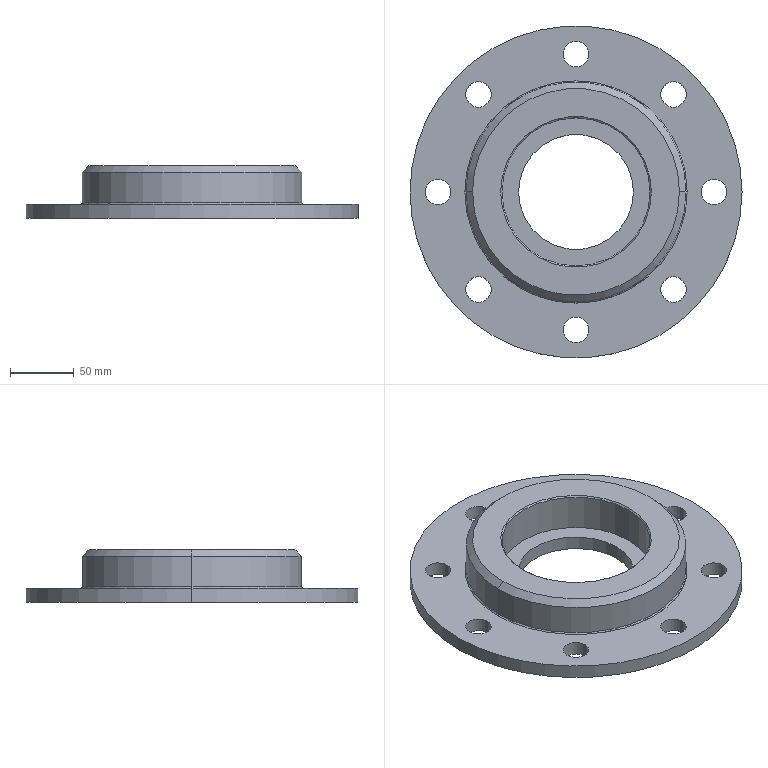Part | SolidWorks | features ICE 3, Chamfer 2, CirPattern 1, Extrusion 1, Fillet 1 | 1 solid | 34 faces | box 260 x 260 x 41 mm | volume 859714 mm3 | cylinder 24 | cone 4 | plane 4 | torus 2 | commonest cylinder face diameters 20 x16 90 x2 116 x2 172 x2 260 x2
STEP:
#1=CARTESIAN_POINT('',(-45.,0.,0.));
#2=VERTEX_POINT('',#1);
#3=CARTESIAN_POINT('',(45.,0.,0.));
#4=VERTEX_POINT('',#3);
#5=CARTESIAN_POINT('',(0.,0.,0.));
#6=DIRECTION('',(0.,0.,1.));
#7=DIRECTION('',(1.,0.,0.));
#8=AXIS2_PLACEMENT_3D('',#5,#6,#7);
#9=CIRCLE('',#8,45.);
#10=EDGE_CURVE('',#2,#4,#9,.T.);
#11=ORIENTED_EDGE('',*,*,#10,.F.);
#12=CARTESIAN_POINT('',(-45.,0.,11.));
#13=VERTEX_POINT('',#12);
#14=CARTESIAN_POINT('',(-45.,0.,0.));
#15=DIRECTION('',(0.,0.,1.));
#16=VECTOR('',#15,1000.);
#17=LINE('',#14,#16);
#18=EDGE_CURVE('',#2,#13,#17,.T.);
#19=ORIENTED_EDGE('',*,*,#18,.T.);
#20=CARTESIAN_POINT('',(45.,0.,11.));
#21=VERTEX_POINT('',#20);
#22=CARTESIAN_POINT('',(0.,0.,11.));
#23=DIRECTION('',(0.,0.,1.));
#24=DIRECTION('',(1.,0.,0.));
#25=AXIS2_PLACEMENT_3D('',#22,#23,#24);
#26=CIRCLE('',#25,45.);
#27=EDGE_CURVE('',#13,#21,#26,.T.);
#28=ORIENTED_EDGE('',*,*,#27,.T.);
#29=CARTESIAN_POINT('',(45.,0.,0.));
#30=DIRECTION('',(0.,0.,1.));
#31=VECTOR('',#30,1000.);
#32=LINE('',#29,#31);
#33=EDGE_CURVE('',#4,#21,#32,.T.);
#34=ORIENTED_EDGE('',*,*,#33,.F.);
#35=EDGE_LOOP('',(#11,#19,#28,#34));
#36=FACE_OUTER_BOUND('',#35,.T.);
#37=CARTESIAN_POINT('',(0.,0.,0.));
#38=DIRECTION('',(0.,0.,1.));
#39=DIRECTION('',(1.,0.,0.));
#40=AXIS2_PLACEMENT_3D('',#37,#38,#39);
#41=CYLINDRICAL_SURFACE('',#40,45.);
#42=ADVANCED_FACE('',(#36),#41,.F.);
#43=CARTESIAN_POINT('',(118.,0.,11.));
#44=VERTEX_POINT('',#43);
#45=CARTESIAN_POINT('',(98.,0.,11.));
#46=VERTEX_POINT('',#45);
#47=CARTESIAN_POINT('',(108.,0.,11.));
#48=DIRECTION('',(0.,0.,-1.));
#49=DIRECTION('',(1.,0.,0.));
#50=AXIS2_PLACEMENT_3D('',#47,#48,#49);
#51=CIRCLE('',#50,10.);
#52=EDGE_CURVE('',#44,#46,#51,.T.);
#53=ORIENTED_EDGE('',*,*,#52,.F.);
#54=CARTESIAN_POINT('',(118.,0.,0.));
#55=VERTEX_POINT('',#54);
#56=CARTESIAN_POINT('',(118.,0.,41.001));
#57=DIRECTION('',(0.,0.,-1.));
#58=VECTOR('',#57,1000.);
#59=LINE('',#56,#58);
#60=EDGE_CURVE('',#44,#55,#59,.T.);
#61=ORIENTED_EDGE('',*,*,#60,.T.);
#62=CARTESIAN_POINT('',(98.,0.,0.));
#63=VERTEX_POINT('',#62);
#64=CARTESIAN_POINT('',(108.,0.,0.));
#65=DIRECTION('',(0.,0.,-1.));
#66=DIRECTION('',(0.,1.,0.));
#67=AXIS2_PLACEMENT_3D('',#64,#65,#66);
#68=CIRCLE('',#67,10.);
#69=EDGE_CURVE('',#55,#63,#68,.T.);
#70=ORIENTED_EDGE('',*,*,#69,.T.);
#71=CARTESIAN_POINT('',(98.,0.,41.001));
#72=DIRECTION('',(0.,0.,-1.));
#73=VECTOR('',#72,1000.);
#74=LINE('',#71,#73);
#75=EDGE_CURVE('',#46,#63,#74,.T.);
#76=ORIENTED_EDGE('',*,*,#75,.F.);
#77=EDGE_LOOP('',(#53,#61,#70,#76));
#78=FACE_OUTER_BOUND('',#77,.T.);
#79=CARTESIAN_POINT('',(108.,0.,41.001));
#80=DIRECTION('',(0.,0.,-1.));
#81=DIRECTION('',(-1.,0.,0.));
#82=AXIS2_PLACEMENT_3D('',#79,#80,#81);
#83=CYLINDRICAL_SURFACE('',#82,10.);
#84=ADVANCED_FACE('',(#78),#83,.F.);
#85=CARTESIAN_POINT('',(86.368,-76.368,11.));
#86=VERTEX_POINT('',#85);
#87=CARTESIAN_POINT('',(66.368,-76.368,11.));
#88=VERTEX_POINT('',#87);
#89=CARTESIAN_POINT('',(76.368,-76.368,11.));
#90=DIRECTION('',(0.,0.,-1.));
#91=DIRECTION('',(1.,0.,0.));
#92=AXIS2_PLACEMENT_3D('',#89,#90,#91);
#93=CIRCLE('',#92,10.);
#94=EDGE_CURVE('',#86,#88,#93,.T.);
#95=ORIENTED_EDGE('',*,*,#94,.F.);
#96=CARTESIAN_POINT('',(86.368,-76.368,0.));
#97=VERTEX_POINT('',#96);
#98=CARTESIAN_POINT('',(86.368,-76.368,41.001));
#99=DIRECTION('',(0.,0.,-1.));
#100=VECTOR('',#99,1000.);
#101=LINE('',#98,#100);
#102=EDGE_CURVE('',#86,#97,#101,.T.);
#103=ORIENTED_EDGE('',*,*,#102,.T.);
#104=CARTESIAN_POINT('',(66.368,-76.368,0.));
#105=VERTEX_POINT('',#104);
#106=CARTESIAN_POINT('',(76.368,-76.368,0.));
#107=DIRECTION('',(0.,0.,-1.));
#108=DIRECTION('',(0.7071,0.7071,0.));
#109=AXIS2_PLACEMENT_3D('',#106,#107,#108);
#110=CIRCLE('',#109,10.);
#111=EDGE_CURVE('',#97,#105,#110,.T.);
#112=ORIENTED_EDGE('',*,*,#111,.T.);
#113=CARTESIAN_POINT('',(66.368,-76.368,41.001));
#114=DIRECTION('',(0.,0.,-1.));
#115=VECTOR('',#114,1000.);
#116=LINE('',#113,#115);
#117=EDGE_CURVE('',#88,#105,#116,.T.);
#118=ORIENTED_EDGE('',*,*,#117,.F.);
#119=EDGE_LOOP('',(#95,#103,#112,#118));
#120=FACE_OUTER_BOUND('',#119,.T.);
#121=CARTESIAN_POINT('',(76.368,-76.368,41.001));
#122=DIRECTION('',(0.,0.,-1.));
#123=DIRECTION('',(-1.,0.,0.));
#124=AXIS2_PLACEMENT_3D('',#121,#122,#123);
#125=CYLINDRICAL_SURFACE('',#124,10.);
#126=ADVANCED_FACE('',(#120),#125,.F.);
#127=CARTESIAN_POINT('',(10.,-108.,11.));
#128=VERTEX_POINT('',#127);
#129=CARTESIAN_POINT('',(-10.,-108.,11.));
#130=VERTEX_POINT('',#129);
#131=CARTESIAN_POINT('',(0.,-108.,11.));
#132=DIRECTION('',(0.,0.,-1.));
#133=DIRECTION('',(1.,0.,0.));
#134=AXIS2_PLACEMENT_3D('',#131,#132,#133);
#135=CIRCLE('',#134,10.);
#136=EDGE_CURVE('',#128,#130,#135,.T.);
#137=ORIENTED_EDGE('',*,*,#136,.F.);
#138=CARTESIAN_POINT('',(10.,-108.,0.));
#139=VERTEX_POINT('',#138);
#140=CARTESIAN_POINT('',(10.,-108.,41.001));
#141=DIRECTION('',(0.,0.,-1.));
#142=VECTOR('',#141,1000.);
#143=LINE('',#140,#142);
#144=EDGE_CURVE('',#128,#139,#143,.T.);
#145=ORIENTED_EDGE('',*,*,#144,.T.);
#146=CARTESIAN_POINT('',(-10.,-108.,0.));
#147=VERTEX_POINT('',#146);
#148=CARTESIAN_POINT('',(0.,-108.,0.));
#149=DIRECTION('',(0.,0.,-1.));
#150=DIRECTION('',(1.,0.,0.));
#151=AXIS2_PLACEMENT_3D('',#148,#149,#150);
#152=CIRCLE('',#151,10.);
#153=EDGE_CURVE('',#139,#147,#152,.T.);
#154=ORIENTED_EDGE('',*,*,#153,.T.);
#155=CARTESIAN_POINT('',(-10.,-108.,41.001));
#156=DIRECTION('',(0.,0.,-1.));
#157=VECTOR('',#156,1000.);
#158=LINE('',#155,#157);
#159=EDGE_CURVE('',#130,#147,#158,.T.);
#160=ORIENTED_EDGE('',*,*,#159,.F.);
#161=EDGE_LOOP('',(#137,#145,#154,#160));
#162=FACE_OUTER_BOUND('',#161,.T.);
#163=CARTESIAN_POINT('',(0.,-108.,41.001));
#164=DIRECTION('',(0.,0.,-1.));
#165=DIRECTION('',(-1.,0.,0.));
#166=AXIS2_PLACEMENT_3D('',#163,#164,#165);
#167=CYLINDRICAL_SURFACE('',#166,10.);
#168=ADVANCED_FACE('',(#162),#167,.F.);
#169=CARTESIAN_POINT('',(-66.368,-76.368,11.));
#170=VERTEX_POINT('',#169);
#171=CARTESIAN_POINT('',(-86.368,-76.368,11.));
#172=VERTEX_POINT('',#171);
#173=CARTESIAN_POINT('',(-76.368,-76.368,11.));
#174=DIRECTION('',(0.,0.,-1.));
#175=DIRECTION('',(1.,0.,0.));
#176=AXIS2_PLACEMENT_3D('',#173,#174,#175);
#177=CIRCLE('',#176,10.);
#178=EDGE_CURVE('',#170,#172,#177,.T.);
#179=ORIENTED_EDGE('',*,*,#178,.F.);
#180=CARTESIAN_POINT('',(-66.368,-76.368,0.));
#181=VERTEX_POINT('',#180);
#182=CARTESIAN_POINT('',(-66.368,-76.368,41.001));
#183=DIRECTION('',(0.,0.,-1.));
#184=VECTOR('',#183,1000.);
#185=LINE('',#182,#184);
#186=EDGE_CURVE('',#170,#181,#185,.T.);
#187=ORIENTED_EDGE('',*,*,#186,.T.);
#188=CARTESIAN_POINT('',(-86.368,-76.368,0.));
#189=VERTEX_POINT('',#188);
#190=CARTESIAN_POINT('',(-76.368,-76.368,0.));
#191=DIRECTION('',(0.,0.,-1.));
#192=DIRECTION('',(0.7071,-0.7071,0.));
#193=AXIS2_PLACEMENT_3D('',#190,#191,#192);
#194=CIRCLE('',#193,10.);
#195=EDGE_CURVE('',#181,#189,#194,.T.);
#196=ORIENTED_EDGE('',*,*,#195,.T.);
#197=CARTESIAN_POINT('',(-86.368,-76.368,41.001));
#198=DIRECTION('',(0.,0.,-1.));
#199=VECTOR('',#198,1000.);
#200=LINE('',#197,#199);
#201=EDGE_CURVE('',#172,#189,#200,.T.);
#202=ORIENTED_EDGE('',*,*,#201,.F.);
#203=EDGE_LOOP('',(#179,#187,#196,#202));
#204=FACE_OUTER_BOUND('',#203,.T.);
#205=CARTESIAN_POINT('',(-76.368,-76.368,41.001));
#206=DIRECTION('',(0.,0.,-1.));
#207=DIRECTION('',(-1.,0.,0.));
#208=AXIS2_PLACEMENT_3D('',#205,#206,#207);
#209=CYLINDRICAL_SURFACE('',#208,10.);
#210=ADVANCED_FACE('',(#204),#209,.F.);
#211=CARTESIAN_POINT('',(-98.,0.,11.));
#212=VERTEX_POINT('',#211);
#213=CARTESIAN_POINT('',(-118.,0.,11.));
#214=VERTEX_POINT('',#213);
#215=CARTESIAN_POINT('',(-108.,0.,11.));
#216=DIRECTION('',(0.,0.,-1.));
#217=DIRECTION('',(1.,0.,0.));
#218=AXIS2_PLACEMENT_3D('',#215,#216,#217);
#219=CIRCLE('',#218,10.);
#220=EDGE_CURVE('',#212,#214,#219,.T.);
#221=ORIENTED_EDGE('',*,*,#220,.F.);
#222=CARTESIAN_POINT('',(-98.,0.,0.));
#223=VERTEX_POINT('',#222);
#224=CARTESIAN_POINT('',(-98.,0.,41.001));
#225=DIRECTION('',(0.,0.,-1.));
#226=VECTOR('',#225,1000.);
#227=LINE('',#224,#226);
#228=EDGE_CURVE('',#212,#223,#227,.T.);
#229=ORIENTED_EDGE('',*,*,#228,.T.);
#230=CARTESIAN_POINT('',(-118.,0.,0.));
#231=VERTEX_POINT('',#230);
#232=CARTESIAN_POINT('',(-108.,0.,0.));
#233=DIRECTION('',(0.,0.,-1.));
#234=DIRECTION('',(0.,-1.,0.));
#235=AXIS2_PLACEMENT_3D('',#232,#233,#234);
#236=CIRCLE('',#235,10.);
#237=EDGE_CURVE('',#223,#231,#236,.T.);
#238=ORIENTED_EDGE('',*,*,#237,.T.);
#239=CARTESIAN_POINT('',(-118.,0.,41.001));
#240=DIRECTION('',(0.,0.,-1.));
#241=VECTOR('',#240,1000.);
#242=LINE('',#239,#241);
#243=EDGE_CURVE('',#214,#231,#242,.T.);
#244=ORIENTED_EDGE('',*,*,#243,.F.);
#245=EDGE_LOOP('',(#221,#229,#238,#244));
#246=FACE_OUTER_BOUND('',#245,.T.);
#247=CARTESIAN_POINT('',(-108.,0.,41.001));
#248=DIRECTION('',(0.,0.,-1.));
#249=DIRECTION('',(-1.,0.,0.));
#250=AXIS2_PLACEMENT_3D('',#247,#248,#249);
#251=CYLINDRICAL_SURFACE('',#250,10.);
#252=ADVANCED_FACE('',(#246),#251,.F.);
#253=CARTESIAN_POINT('',(-66.368,76.368,11.));
#254=VERTEX_POINT('',#253);
#255=CARTESIAN_POINT('',(-86.368,76.368,11.));
#256=VERTEX_POINT('',#255);
#257=CARTESIAN_POINT('',(-76.368,76.368,11.));
#258=DIRECTION('',(0.,0.,-1.));
#259=DIRECTION('',(1.,0.,0.));
#260=AXIS2_PLACEMENT_3D('',#257,#258,#259);
#261=CIRCLE('',#260,10.);
#262=EDGE_CURVE('',#254,#256,#261,.T.);
#263=ORIENTED_EDGE('',*,*,#262,.F.);
#264=CARTESIAN_POINT('',(-66.368,76.368,0.));
#265=VERTEX_POINT('',#264);
#266=CARTESIAN_POINT('',(-66.368,76.368,41.001));
#267=DIRECTION('',(0.,0.,-1.));
#268=VECTOR('',#267,1000.);
#269=LINE('',#266,#268);
#270=EDGE_CURVE('',#254,#265,#269,.T.);
#271=ORIENTED_EDGE('',*,*,#270,.T.);
#272=CARTESIAN_POINT('',(-86.368,76.368,0.));
#273=VERTEX_POINT('',#272);
#274=CARTESIAN_POINT('',(-76.368,76.368,0.));
#275=DIRECTION('',(0.,0.,-1.));
#276=DIRECTION('',(-0.7071,-0.7071,0.));
#277=AXIS2_PLACEMENT_3D('',#274,#275,#276);
#278=CIRCLE('',#277,10.);
#279=EDGE_CURVE('',#265,#273,#278,.T.);
#280=ORIENTED_EDGE('',*,*,#279,.T.);
#281=CARTESIAN_POINT('',(-86.368,76.368,41.001));
#282=DIRECTION('',(0.,0.,-1.));
#283=VECTOR('',#282,1000.);
#284=LINE('',#281,#283);
#285=EDGE_CURVE('',#256,#273,#284,.T.);
#286=ORIENTED_EDGE('',*,*,#285,.F.);
#287=EDGE_LOOP('',(#263,#271,#280,#286));
#288=FACE_OUTER_BOUND('',#287,.T.);
#289=CARTESIAN_POINT('',(-76.368,76.368,41.001));
#290=DIRECTION('',(0.,0.,-1.));
#291=DIRECTION('',(-1.,0.,0.));
#292=AXIS2_PLACEMENT_3D('',#289,#290,#291);
#293=CYLINDRICAL_SURFACE('',#292,10.);
#294=ADVANCED_FACE('',(#288),#293,.F.);
#295=CARTESIAN_POINT('',(86.368,76.368,11.));
#296=VERTEX_POINT('',#295);
#297=CARTESIAN_POINT('',(66.368,76.368,11.));
#298=VERTEX_POINT('',#297);
#299=CARTESIAN_POINT('',(76.368,76.368,11.));
#300=DIRECTION('',(0.,0.,-1.));
#301=DIRECTION('',(1.,0.,0.));
#302=AXIS2_PLACEMENT_3D('',#299,#300,#301);
#303=CIRCLE('',#302,10.);
#304=EDGE_CURVE('',#296,#298,#303,.T.);
#305=ORIENTED_EDGE('',*,*,#304,.F.);
#306=CARTESIAN_POINT('',(86.368,76.368,0.));
#307=VERTEX_POINT('',#306);
#308=CARTESIAN_POINT('',(86.368,76.368,41.001));
#309=DIRECTION('',(0.,0.,-1.));
#310=VECTOR('',#309,1000.);
#311=LINE('',#308,#310);
#312=EDGE_CURVE('',#296,#307,#311,.T.);
#313=ORIENTED_EDGE('',*,*,#312,.T.);
#314=CARTESIAN_POINT('',(66.368,76.368,0.));
#315=VERTEX_POINT('',#314);
#316=CARTESIAN_POINT('',(76.368,76.368,0.));
#317=DIRECTION('',(0.,0.,-1.));
#318=DIRECTION('',(-0.7071,0.7071,0.));
#319=AXIS2_PLACEMENT_3D('',#316,#317,#318);
#320=CIRCLE('',#319,10.);
#321=EDGE_CURVE('',#307,#315,#320,.T.);
#322=ORIENTED_EDGE('',*,*,#321,.T.);
#323=CARTESIAN_POINT('',(66.368,76.368,41.001));
#324=DIRECTION('',(0.,0.,-1.));
#325=VECTOR('',#324,1000.);
#326=LINE('',#323,#325);
#327=EDGE_CURVE('',#298,#315,#326,.T.);
#328=ORIENTED_EDGE('',*,*,#327,.F.);
#329=EDGE_LOOP('',(#305,#313,#322,#328));
#330=FACE_OUTER_BOUND('',#329,.T.);
#331=CARTESIAN_POINT('',(76.368,76.368,41.001));
#332=DIRECTION('',(0.,0.,-1.));
#333=DIRECTION('',(-1.,0.,0.));
#334=AXIS2_PLACEMENT_3D('',#331,#332,#333);
#335=CYLINDRICAL_SURFACE('',#334,10.);
#336=ADVANCED_FACE('',(#330),#335,.F.);
#337=CARTESIAN_POINT('',(10.,108.,11.));
#338=VERTEX_POINT('',#337);
#339=CARTESIAN_POINT('',(-10.,108.,11.));
#340=VERTEX_POINT('',#339);
#341=CARTESIAN_POINT('',(0.,108.,11.));
#342=DIRECTION('',(0.,0.,-1.));
#343=DIRECTION('',(1.,0.,0.));
#344=AXIS2_PLACEMENT_3D('',#341,#342,#343);
#345=CIRCLE('',#344,10.);
#346=EDGE_CURVE('',#338,#340,#345,.T.);
#347=ORIENTED_EDGE('',*,*,#346,.F.);
#348=CARTESIAN_POINT('',(10.,108.,0.));
#349=VERTEX_POINT('',#348);
#350=CARTESIAN_POINT('',(10.,108.,41.001));
#351=DIRECTION('',(0.,0.,-1.));
#352=VECTOR('',#351,1000.);
#353=LINE('',#350,#352);
#354=EDGE_CURVE('',#338,#349,#353,.T.);
#355=ORIENTED_EDGE('',*,*,#354,.T.);
#356=CARTESIAN_POINT('',(-10.,108.,0.));
#357=VERTEX_POINT('',#356);
#358=CARTESIAN_POINT('',(0.,108.,0.));
#359=DIRECTION('',(0.,0.,-1.));
#360=DIRECTION('',(-1.,0.,0.));
#361=AXIS2_PLACEMENT_3D('',#358,#359,#360);
#362=CIRCLE('',#361,10.);
#363=EDGE_CURVE('',#349,#357,#362,.T.);
#364=ORIENTED_EDGE('',*,*,#363,.T.);
#365=CARTESIAN_POINT('',(-10.,108.,41.001));
#366=DIRECTION('',(0.,0.,-1.));
#367=VECTOR('',#366,1000.);
#368=LINE('',#365,#367);
#369=EDGE_CURVE('',#340,#357,#368,.T.);
#370=ORIENTED_EDGE('',*,*,#369,.F.);
#371=EDGE_LOOP('',(#347,#355,#364,#370));
#372=FACE_OUTER_BOUND('',#371,.T.);
#373=CARTESIAN_POINT('',(0.,108.,41.001));
#374=DIRECTION('',(0.,0.,-1.));
#375=DIRECTION('',(-1.,0.,0.));
#376=AXIS2_PLACEMENT_3D('',#373,#374,#375);
#377=CYLINDRICAL_SURFACE('',#376,10.);
#378=ADVANCED_FACE('',(#372),#377,.F.);
#379=CARTESIAN_POINT('',(81.,0.,41.));
#380=VERTEX_POINT('',#379);
#381=CARTESIAN_POINT('',(-81.,0.,41.));
#382=VERTEX_POINT('',#381);
#383=CARTESIAN_POINT('',(0.,0.,41.));
#384=DIRECTION('',(0.,0.,1.));
#385=DIRECTION('',(1.,0.,0.));
#386=AXIS2_PLACEMENT_3D('',#383,#384,#385);
#387=CIRCLE('',#386,81.);
#388=EDGE_CURVE('',#380,#382,#387,.T.);
#389=ORIENTED_EDGE('',*,*,#388,.F.);
#390=CARTESIAN_POINT('',(86.,0.,36.));
#391=VERTEX_POINT('',#390);
#392=CARTESIAN_POINT('',(81.,0.,41.));
#393=DIRECTION('',(0.7071,0.,-0.7071));
#394=VECTOR('',#393,1000.);
#395=LINE('',#392,#394);
#396=EDGE_CURVE('',#380,#391,#395,.T.);
#397=ORIENTED_EDGE('',*,*,#396,.T.);
#398=CARTESIAN_POINT('',(-86.,0.,36.));
#399=VERTEX_POINT('',#398);
#400=CARTESIAN_POINT('',(0.,0.,36.));
#401=DIRECTION('',(0.,0.,-1.));
#402=DIRECTION('',(1.,0.,0.));
#403=AXIS2_PLACEMENT_3D('',#400,#401,#402);
#404=CIRCLE('',#403,86.);
#405=EDGE_CURVE('',#399,#391,#404,.T.);
#406=ORIENTED_EDGE('',*,*,#405,.F.);
#407=CARTESIAN_POINT('',(-81.,0.,41.));
#408=DIRECTION('',(-0.7071,0.,-0.7071));
#409=VECTOR('',#408,1000.);
#410=LINE('',#407,#409);
#411=EDGE_CURVE('',#382,#399,#410,.T.);
#412=ORIENTED_EDGE('',*,*,#411,.F.);
#413=EDGE_LOOP('',(#389,#397,#406,#412));
#414=FACE_OUTER_BOUND('',#413,.T.);
#415=CARTESIAN_POINT('',(0.,0.,41.));
#416=DIRECTION('',(0.,0.,-1.));
#417=DIRECTION('',(-1.,0.,0.));
#418=AXIS2_PLACEMENT_3D('',#415,#416,#417);
#419=CONICAL_SURFACE('',#418,81.,0.7854);
#420=ADVANCED_FACE('',(#414),#419,.T.);
#421=CARTESIAN_POINT('',(-58.,0.,40.));
#422=VERTEX_POINT('',#421);
#423=CARTESIAN_POINT('',(58.,0.,40.));
#424=VERTEX_POINT('',#423);
#425=CARTESIAN_POINT('',(0.,0.,40.));
#426=DIRECTION('',(0.,0.,1.));
#427=DIRECTION('',(1.,0.,0.));
#428=AXIS2_PLACEMENT_3D('',#425,#426,#427);
#429=CIRCLE('',#428,58.);
#430=EDGE_CURVE('',#422,#424,#429,.T.);
#431=ORIENTED_EDGE('',*,*,#430,.F.);
#432=CARTESIAN_POINT('',(-59.,0.,41.));
#433=VERTEX_POINT('',#432);
#434=CARTESIAN_POINT('',(-58.,0.,40.));
#435=DIRECTION('',(-0.7071,0.,0.7071));
#436=VECTOR('',#435,1000.);
#437=LINE('',#434,#436);
#438=EDGE_CURVE('',#422,#433,#437,.T.);
#439=ORIENTED_EDGE('',*,*,#438,.T.);
#440=CARTESIAN_POINT('',(59.,0.,41.));
#441=VERTEX_POINT('',#440);
#442=CARTESIAN_POINT('',(0.,0.,41.));
#443=DIRECTION('',(0.,0.,-1.));
#444=DIRECTION('',(1.,0.,0.));
#445=AXIS2_PLACEMENT_3D('',#442,#443,#444);
#446=CIRCLE('',#445,59.);
#447=EDGE_CURVE('',#441,#433,#446,.T.);
#448=ORIENTED_EDGE('',*,*,#447,.F.);
#449=CARTESIAN_POINT('',(58.,0.,40.));
#450=DIRECTION('',(0.7071,0.,0.7071));
#451=VECTOR('',#450,1000.);
#452=LINE('',#449,#451);
#453=EDGE_CURVE('',#424,#441,#452,.T.);
#454=ORIENTED_EDGE('',*,*,#453,.F.);
#455=EDGE_LOOP('',(#431,#439,#448,#454));
#456=FACE_OUTER_BOUND('',#455,.T.);
#457=CARTESIAN_POINT('',(0.,0.,40.));
#458=DIRECTION('',(0.,0.,1.));
#459=DIRECTION('',(1.,0.,0.));
#460=AXIS2_PLACEMENT_3D('',#457,#458,#459);
#461=CONICAL_SURFACE('',#460,58.,0.7854);
#462=ADVANCED_FACE('',(#456),#461,.F.);
#463=CARTESIAN_POINT('',(-86.,0.,12.));
#464=VERTEX_POINT('',#463);
#465=CARTESIAN_POINT('',(86.,0.,12.));
#466=VERTEX_POINT('',#465);
#467=CARTESIAN_POINT('',(0.,0.,12.));
#468=DIRECTION('',(0.,0.,1.));
#469=DIRECTION('',(1.,0.,0.));
#470=AXIS2_PLACEMENT_3D('',#467,#468,#469);
#471=CIRCLE('',#470,86.);
#472=EDGE_CURVE('',#464,#466,#471,.T.);
#473=ORIENTED_EDGE('',*,*,#472,.F.);
#474=CARTESIAN_POINT('',(-87.,0.,11.));
#475=VERTEX_POINT('',#474);
#476=CARTESIAN_POINT('',(-87.,0.,12.));
#477=DIRECTION('',(0.,1.,0.));
#478=DIRECTION('',(-1.,0.,0.));
#479=AXIS2_PLACEMENT_3D('',#476,#477,#478);
#480=CIRCLE('',#479,1.);
#481=EDGE_CURVE('',#464,#475,#480,.T.);
#482=ORIENTED_EDGE('',*,*,#481,.T.);
#483=CARTESIAN_POINT('',(87.,0.,11.));
#484=VERTEX_POINT('',#483);
#485=CARTESIAN_POINT('',(0.,0.,11.));
#486=DIRECTION('',(0.,0.,-1.));
#487=DIRECTION('',(1.,0.,0.));
#488=AXIS2_PLACEMENT_3D('',#485,#486,#487);
#489=CIRCLE('',#488,87.);
#490=EDGE_CURVE('',#484,#475,#489,.T.);
#491=ORIENTED_EDGE('',*,*,#490,.F.);
#492=CARTESIAN_POINT('',(87.,0.,12.));
#493=DIRECTION('',(0.,-1.,0.));
#494=DIRECTION('',(0.,0.,-1.));
#495=AXIS2_PLACEMENT_3D('',#492,#493,#494);
#496=CIRCLE('',#495,1.);
#497=EDGE_CURVE('',#466,#484,#496,.T.);
#498=ORIENTED_EDGE('',*,*,#497,.F.);
#499=EDGE_LOOP('',(#473,#482,#491,#498));
#500=FACE_OUTER_BOUND('',#499,.T.);
#501=CARTESIAN_POINT('',(0.,0.,12.));
#502=DIRECTION('',(0.,0.,1.));
#503=DIRECTION('',(1.,0.,0.));
#504=AXIS2_PLACEMENT_3D('',#501,#502,#503);
#505=TOROIDAL_SURFACE('',#504,87.,1.);
#506=ADVANCED_FACE('',(#500),#505,.F.);
#507=ORIENTED_EDGE('',*,*,#430,.T.);
#508=CARTESIAN_POINT('',(58.,0.,11.));
#509=VERTEX_POINT('',#508);
#510=CARTESIAN_POINT('',(58.,0.,41.));
#511=DIRECTION('',(0.,0.,-1.));
#512=VECTOR('',#511,1000.);
#513=LINE('',#510,#512);
#514=EDGE_CURVE('',#424,#509,#513,.T.);
#515=ORIENTED_EDGE('',*,*,#514,.T.);
#516=CARTESIAN_POINT('',(-58.,0.,11.));
#517=VERTEX_POINT('',#516);
#518=CARTESIAN_POINT('',(0.,0.,11.));
#519=DIRECTION('',(0.,0.,-1.));
#520=DIRECTION('',(1.,0.,0.));
#521=AXIS2_PLACEMENT_3D('',#518,#519,#520);
#522=CIRCLE('',#521,58.);
#523=EDGE_CURVE('',#509,#517,#522,.T.);
#524=ORIENTED_EDGE('',*,*,#523,.T.);
#525=CARTESIAN_POINT('',(-58.,0.,41.));
#526=DIRECTION('',(0.,0.,-1.));
#527=VECTOR('',#526,1000.);
#528=LINE('',#525,#527);
#529=EDGE_CURVE('',#422,#517,#528,.T.);
#530=ORIENTED_EDGE('',*,*,#529,.F.);
#531=EDGE_LOOP('',(#507,#515,#524,#530));
#532=FACE_OUTER_BOUND('',#531,.T.);
#533=CARTESIAN_POINT('',(0.,0.,41.));
#534=DIRECTION('',(0.,0.,-1.));
#535=DIRECTION('',(-1.,0.,0.));
#536=AXIS2_PLACEMENT_3D('',#533,#534,#535);
#537=CYLINDRICAL_SURFACE('',#536,58.);
#538=ADVANCED_FACE('',(#532),#537,.F.);
#539=ORIENTED_EDGE('',*,*,#405,.T.);
#540=CARTESIAN_POINT('',(86.,0.,41.));
#541=DIRECTION('',(0.,0.,-1.));
#542=VECTOR('',#541,1000.);
#543=LINE('',#540,#542);
#544=EDGE_CURVE('',#391,#466,#543,.T.);
#545=ORIENTED_EDGE('',*,*,#544,.T.);
#546=CARTESIAN_POINT('',(0.,0.,12.));
#547=DIRECTION('',(0.,0.,1.));
#548=DIRECTION('',(1.,0.,0.));
#549=AXIS2_PLACEMENT_3D('',#546,#547,#548);
#550=CIRCLE('',#549,86.);
#551=EDGE_CURVE('',#466,#464,#550,.T.);
#552=ORIENTED_EDGE('',*,*,#551,.T.);
#553=CARTESIAN_POINT('',(-86.,0.,41.));
#554=DIRECTION('',(0.,0.,-1.));
#555=VECTOR('',#554,1000.);
#556=LINE('',#553,#555);
#557=EDGE_CURVE('',#399,#464,#556,.T.);
#558=ORIENTED_EDGE('',*,*,#557,.F.);
#559=EDGE_LOOP('',(#539,#545,#552,#558));
#560=FACE_OUTER_BOUND('',#559,.T.);
#561=CARTESIAN_POINT('',(0.,0.,41.));
#562=DIRECTION('',(0.,0.,-1.));
#563=DIRECTION('',(-1.,0.,0.));
#564=AXIS2_PLACEMENT_3D('',#561,#562,#563);
#565=CYLINDRICAL_SURFACE('',#564,86.);
#566=ADVANCED_FACE('',(#560),#565,.T.);
#567=CARTESIAN_POINT('',(130.,0.,11.));
#568=VERTEX_POINT('',#567);
#569=CARTESIAN_POINT('',(-130.,0.,11.));
#570=VERTEX_POINT('',#569);
#571=CARTESIAN_POINT('',(0.,0.,11.));
#572=DIRECTION('',(0.,0.,1.));
#573=DIRECTION('',(1.,0.,0.));
#574=AXIS2_PLACEMENT_3D('',#571,#572,#573);
#575=CIRCLE('',#574,130.);
#576=EDGE_CURVE('',#568,#570,#575,.T.);
#577=ORIENTED_EDGE('',*,*,#576,.F.);
#578=CARTESIAN_POINT('',(130.,0.,0.));
#579=VERTEX_POINT('',#578);
#580=CARTESIAN_POINT('',(130.,0.,11.));
#581=DIRECTION('',(0.,0.,-1.));
#582=VECTOR('',#581,1000.);
#583=LINE('',#580,#582);
#584=EDGE_CURVE('',#568,#579,#583,.T.);
#585=ORIENTED_EDGE('',*,*,#584,.T.);
#586=CARTESIAN_POINT('',(-130.,0.,0.));
#587=VERTEX_POINT('',#586);
#588=CARTESIAN_POINT('',(0.,0.,0.));
#589=DIRECTION('',(0.,0.,1.));
#590=DIRECTION('',(1.,0.,0.));
#591=AXIS2_PLACEMENT_3D('',#588,#589,#590);
#592=CIRCLE('',#591,130.);
#593=EDGE_CURVE('',#579,#587,#592,.T.);
#594=ORIENTED_EDGE('',*,*,#593,.T.);
#595=CARTESIAN_POINT('',(-130.,0.,11.));
#596=DIRECTION('',(0.,0.,-1.));
#597=VECTOR('',#596,1000.);
#598=LINE('',#595,#597);
#599=EDGE_CURVE('',#570,#587,#598,.T.);
#600=ORIENTED_EDGE('',*,*,#599,.F.);
#601=EDGE_LOOP('',(#577,#585,#594,#600));
#602=FACE_OUTER_BOUND('',#601,.T.);
#603=CARTESIAN_POINT('',(0.,0.,11.));
#604=DIRECTION('',(0.,0.,-1.));
#605=DIRECTION('',(-1.,0.,0.));
#606=AXIS2_PLACEMENT_3D('',#603,#604,#605);
#607=CYLINDRICAL_SURFACE('',#606,130.);
#608=ADVANCED_FACE('',(#602),#607,.T.);
#609=ORIENTED_EDGE('',*,*,#584,.F.);
#610=CARTESIAN_POINT('',(0.,0.,11.));
#611=DIRECTION('',(0.,0.,1.));
#612=DIRECTION('',(1.,0.,0.));
#613=AXIS2_PLACEMENT_3D('',#610,#611,#612);
#614=CIRCLE('',#613,130.);
#615=EDGE_CURVE('',#570,#568,#614,.T.);
#616=ORIENTED_EDGE('',*,*,#615,.F.);
#617=ORIENTED_EDGE('',*,*,#599,.T.);
#618=CARTESIAN_POINT('',(0.,0.,0.));
#619=DIRECTION('',(0.,0.,1.));
#620=DIRECTION('',(1.,0.,0.));
#621=AXIS2_PLACEMENT_3D('',#618,#619,#620);
#622=CIRCLE('',#621,130.);
#623=EDGE_CURVE('',#587,#579,#622,.T.);
#624=ORIENTED_EDGE('',*,*,#623,.T.);
#625=EDGE_LOOP('',(#609,#616,#617,#624));
#626=FACE_OUTER_BOUND('',#625,.T.);
#627=CARTESIAN_POINT('',(0.,0.,11.));
#628=DIRECTION('',(0.,0.,-1.));
#629=DIRECTION('',(-1.,0.,0.));
#630=AXIS2_PLACEMENT_3D('',#627,#628,#629);
#631=CYLINDRICAL_SURFACE('',#630,130.);
#632=ADVANCED_FACE('',(#626),#631,.T.);
#633=CARTESIAN_POINT('',(108.,0.,11.));
#634=DIRECTION('',(0.,0.,-1.));
#635=DIRECTION('',(1.,0.,0.));
#636=AXIS2_PLACEMENT_3D('',#633,#634,#635);
#637=CIRCLE('',#636,10.);
#638=EDGE_CURVE('',#46,#44,#637,.T.);
#639=ORIENTED_EDGE('',*,*,#638,.T.);
#640=ORIENTED_EDGE('',*,*,#52,.T.);
#641=EDGE_LOOP('',(#639,#640));
#642=FACE_BOUND('',#641,.T.);
#643=CARTESIAN_POINT('',(76.368,-76.368,11.));
#644=DIRECTION('',(0.,0.,-1.));
#645=DIRECTION('',(1.,0.,0.));
#646=AXIS2_PLACEMENT_3D('',#643,#644,#645);
#647=CIRCLE('',#646,10.);
#648=EDGE_CURVE('',#88,#86,#647,.T.);
#649=ORIENTED_EDGE('',*,*,#648,.T.);
#650=ORIENTED_EDGE('',*,*,#94,.T.);
#651=EDGE_LOOP('',(#649,#650));
#652=FACE_BOUND('',#651,.T.);
#653=CARTESIAN_POINT('',(0.,-108.,11.));
#654=DIRECTION('',(0.,0.,-1.));
#655=DIRECTION('',(1.,0.,0.));
#656=AXIS2_PLACEMENT_3D('',#653,#654,#655);
#657=CIRCLE('',#656,10.);
#658=EDGE_CURVE('',#130,#128,#657,.T.);
#659=ORIENTED_EDGE('',*,*,#658,.T.);
#660=ORIENTED_EDGE('',*,*,#136,.T.);
#661=EDGE_LOOP('',(#659,#660));
#662=FACE_BOUND('',#661,.T.);
#663=CARTESIAN_POINT('',(-76.368,-76.368,11.));
#664=DIRECTION('',(0.,0.,-1.));
#665=DIRECTION('',(1.,0.,0.));
#666=AXIS2_PLACEMENT_3D('',#663,#664,#665);
#667=CIRCLE('',#666,10.);
#668=EDGE_CURVE('',#172,#170,#667,.T.);
#669=ORIENTED_EDGE('',*,*,#668,.T.);
#670=ORIENTED_EDGE('',*,*,#178,.T.);
#671=EDGE_LOOP('',(#669,#670));
#672=FACE_BOUND('',#671,.T.);
#673=CARTESIAN_POINT('',(-108.,0.,11.));
#674=DIRECTION('',(0.,0.,-1.));
#675=DIRECTION('',(1.,0.,0.));
#676=AXIS2_PLACEMENT_3D('',#673,#674,#675);
#677=CIRCLE('',#676,10.);
#678=EDGE_CURVE('',#214,#212,#677,.T.);
#679=ORIENTED_EDGE('',*,*,#678,.T.);
#680=ORIENTED_EDGE('',*,*,#220,.T.);
#681=EDGE_LOOP('',(#679,#680));
#682=FACE_BOUND('',#681,.T.);
#683=CARTESIAN_POINT('',(-76.368,76.368,11.));
#684=DIRECTION('',(0.,0.,-1.));
#685=DIRECTION('',(1.,0.,0.));
#686=AXIS2_PLACEMENT_3D('',#683,#684,#685);
#687=CIRCLE('',#686,10.);
#688=EDGE_CURVE('',#256,#254,#687,.T.);
#689=ORIENTED_EDGE('',*,*,#688,.T.);
#690=ORIENTED_EDGE('',*,*,#262,.T.);
#691=EDGE_LOOP('',(#689,#690));
#692=FACE_BOUND('',#691,.T.);
#693=CARTESIAN_POINT('',(76.368,76.368,11.));
#694=DIRECTION('',(0.,0.,-1.));
#695=DIRECTION('',(1.,0.,0.));
#696=AXIS2_PLACEMENT_3D('',#693,#694,#695);
#697=CIRCLE('',#696,10.);
#698=EDGE_CURVE('',#298,#296,#697,.T.);
#699=ORIENTED_EDGE('',*,*,#698,.T.);
#700=ORIENTED_EDGE('',*,*,#304,.T.);
#701=EDGE_LOOP('',(#699,#700));
#702=FACE_BOUND('',#701,.T.);
#703=CARTESIAN_POINT('',(0.,108.,11.));
#704=DIRECTION('',(0.,0.,-1.));
#705=DIRECTION('',(1.,0.,0.));
#706=AXIS2_PLACEMENT_3D('',#703,#704,#705);
#707=CIRCLE('',#706,10.);
#708=EDGE_CURVE('',#340,#338,#707,.T.);
#709=ORIENTED_EDGE('',*,*,#708,.T.);
#710=ORIENTED_EDGE('',*,*,#346,.T.);
#711=EDGE_LOOP('',(#709,#710));
#712=FACE_BOUND('',#711,.T.);
#713=ORIENTED_EDGE('',*,*,#490,.T.);
#714=CARTESIAN_POINT('',(0.,0.,11.));
#715=DIRECTION('',(0.,0.,-1.));
#716=DIRECTION('',(1.,0.,0.));
#717=AXIS2_PLACEMENT_3D('',#714,#715,#716);
#718=CIRCLE('',#717,87.);
#719=EDGE_CURVE('',#475,#484,#718,.T.);
#720=ORIENTED_EDGE('',*,*,#719,.T.);
#721=EDGE_LOOP('',(#713,#720));
#722=FACE_BOUND('',#721,.T.);
#723=ORIENTED_EDGE('',*,*,#615,.T.);
#724=ORIENTED_EDGE('',*,*,#576,.T.);
#725=EDGE_LOOP('',(#723,#724));
#726=FACE_OUTER_BOUND('',#725,.T.);
#727=CARTESIAN_POINT('',(0.,0.,11.));
#728=DIRECTION('',(0.,0.,1.));
#729=DIRECTION('',(1.,0.,0.));
#730=AXIS2_PLACEMENT_3D('',#727,#728,#729);
#731=PLANE('',#730);
#732=ADVANCED_FACE('',(#642,#652,#662,#672,#682,#692,#702,#712,#722,#726),#731,.T.);
#733=CARTESIAN_POINT('',(0.,0.,0.));
#734=DIRECTION('',(0.,0.,1.));
#735=DIRECTION('',(1.,0.,0.));
#736=AXIS2_PLACEMENT_3D('',#733,#734,#735);
#737=CIRCLE('',#736,45.);
#738=EDGE_CURVE('',#4,#2,#737,.T.);
#739=ORIENTED_EDGE('',*,*,#738,.T.);
#740=ORIENTED_EDGE('',*,*,#10,.T.);
#741=EDGE_LOOP('',(#739,#740));
#742=FACE_BOUND('',#741,.T.);
#743=CARTESIAN_POINT('',(108.,0.,0.));
#744=DIRECTION('',(0.,0.,-1.));
#745=DIRECTION('',(0.,1.,0.));
#746=AXIS2_PLACEMENT_3D('',#743,#744,#745);
#747=CIRCLE('',#746,10.);
#748=EDGE_CURVE('',#63,#55,#747,.T.);
#749=ORIENTED_EDGE('',*,*,#748,.F.);
#750=ORIENTED_EDGE('',*,*,#69,.F.);
#751=EDGE_LOOP('',(#749,#750));
#752=FACE_BOUND('',#751,.T.);
#753=CARTESIAN_POINT('',(76.368,-76.368,0.));
#754=DIRECTION('',(0.,0.,-1.));
#755=DIRECTION('',(0.7071,0.7071,0.));
#756=AXIS2_PLACEMENT_3D('',#753,#754,#755);
#757=CIRCLE('',#756,10.);
#758=EDGE_CURVE('',#105,#97,#757,.T.);
#759=ORIENTED_EDGE('',*,*,#758,.F.);
#760=ORIENTED_EDGE('',*,*,#111,.F.);
#761=EDGE_LOOP('',(#759,#760));
#762=FACE_BOUND('',#761,.T.);
#763=CARTESIAN_POINT('',(0.,-108.,0.));
#764=DIRECTION('',(0.,0.,-1.));
#765=DIRECTION('',(1.,0.,0.));
#766=AXIS2_PLACEMENT_3D('',#763,#764,#765);
#767=CIRCLE('',#766,10.);
#768=EDGE_CURVE('',#147,#139,#767,.T.);
#769=ORIENTED_EDGE('',*,*,#768,.F.);
#770=ORIENTED_EDGE('',*,*,#153,.F.);
#771=EDGE_LOOP('',(#769,#770));
#772=FACE_BOUND('',#771,.T.);
#773=CARTESIAN_POINT('',(-76.368,-76.368,0.));
#774=DIRECTION('',(0.,0.,-1.));
#775=DIRECTION('',(0.7071,-0.7071,0.));
#776=AXIS2_PLACEMENT_3D('',#773,#774,#775);
#777=CIRCLE('',#776,10.);
#778=EDGE_CURVE('',#189,#181,#777,.T.);
#779=ORIENTED_EDGE('',*,*,#778,.F.);
#780=ORIENTED_EDGE('',*,*,#195,.F.);
#781=EDGE_LOOP('',(#779,#780));
#782=FACE_BOUND('',#781,.T.);
#783=CARTESIAN_POINT('',(-108.,0.,0.));
#784=DIRECTION('',(0.,0.,-1.));
#785=DIRECTION('',(0.,-1.,0.));
#786=AXIS2_PLACEMENT_3D('',#783,#784,#785);
#787=CIRCLE('',#786,10.);
#788=EDGE_CURVE('',#231,#223,#787,.T.);
#789=ORIENTED_EDGE('',*,*,#788,.F.);
#790=ORIENTED_EDGE('',*,*,#237,.F.);
#791=EDGE_LOOP('',(#789,#790));
#792=FACE_BOUND('',#791,.T.);
#793=CARTESIAN_POINT('',(-76.368,76.368,0.));
#794=DIRECTION('',(0.,0.,-1.));
#795=DIRECTION('',(-0.7071,-0.7071,0.));
#796=AXIS2_PLACEMENT_3D('',#793,#794,#795);
#797=CIRCLE('',#796,10.);
#798=EDGE_CURVE('',#273,#265,#797,.T.);
#799=ORIENTED_EDGE('',*,*,#798,.F.);
#800=ORIENTED_EDGE('',*,*,#279,.F.);
#801=EDGE_LOOP('',(#799,#800));
#802=FACE_BOUND('',#801,.T.);
#803=CARTESIAN_POINT('',(76.368,76.368,0.));
#804=DIRECTION('',(0.,0.,-1.));
#805=DIRECTION('',(-0.7071,0.7071,0.));
#806=AXIS2_PLACEMENT_3D('',#803,#804,#805);
#807=CIRCLE('',#806,10.);
#808=EDGE_CURVE('',#315,#307,#807,.T.);
#809=ORIENTED_EDGE('',*,*,#808,.F.);
#810=ORIENTED_EDGE('',*,*,#321,.F.);
#811=EDGE_LOOP('',(#809,#810));
#812=FACE_BOUND('',#811,.T.);
#813=CARTESIAN_POINT('',(0.,108.,0.));
#814=DIRECTION('',(0.,0.,-1.));
#815=DIRECTION('',(-1.,0.,0.));
#816=AXIS2_PLACEMENT_3D('',#813,#814,#815);
#817=CIRCLE('',#816,10.);
#818=EDGE_CURVE('',#357,#349,#817,.T.);
#819=ORIENTED_EDGE('',*,*,#818,.F.);
#820=ORIENTED_EDGE('',*,*,#363,.F.);
#821=EDGE_LOOP('',(#819,#820));
#822=FACE_BOUND('',#821,.T.);
#823=ORIENTED_EDGE('',*,*,#623,.F.);
#824=ORIENTED_EDGE('',*,*,#593,.F.);
#825=EDGE_LOOP('',(#823,#824));
#826=FACE_OUTER_BOUND('',#825,.T.);
#827=CARTESIAN_POINT('',(0.,0.,0.));
#828=DIRECTION('',(0.,0.,1.));
#829=DIRECTION('',(1.,0.,0.));
#830=AXIS2_PLACEMENT_3D('',#827,#828,#829);
#831=PLANE('',#830);
#832=ADVANCED_FACE('',(#742,#752,#762,#772,#782,#792,#802,#812,#822,#826),#831,.F.);
#833=CARTESIAN_POINT('',(0.,0.,41.));
#834=DIRECTION('',(0.,0.,1.));
#835=DIRECTION('',(1.,0.,0.));
#836=AXIS2_PLACEMENT_3D('',#833,#834,#835);
#837=CIRCLE('',#836,81.);
#838=EDGE_CURVE('',#382,#380,#837,.T.);
#839=ORIENTED_EDGE('',*,*,#838,.T.);
#840=ORIENTED_EDGE('',*,*,#388,.T.);
#841=EDGE_LOOP('',(#839,#840));
#842=FACE_OUTER_BOUND('',#841,.T.);
#843=ORIENTED_EDGE('',*,*,#447,.T.);
#844=CARTESIAN_POINT('',(0.,0.,41.));
#845=DIRECTION('',(0.,0.,-1.));
#846=DIRECTION('',(1.,0.,0.));
#847=AXIS2_PLACEMENT_3D('',#844,#845,#846);
#848=CIRCLE('',#847,59.);
#849=EDGE_CURVE('',#433,#441,#848,.T.);
#850=ORIENTED_EDGE('',*,*,#849,.T.);
#851=EDGE_LOOP('',(#843,#850));
#852=FACE_BOUND('',#851,.T.);
#853=CARTESIAN_POINT('',(0.,0.,41.));
#854=DIRECTION('',(0.,0.,1.));
#855=DIRECTION('',(1.,0.,0.));
#856=AXIS2_PLACEMENT_3D('',#853,#854,#855);
#857=PLANE('',#856);
#858=ADVANCED_FACE('',(#842,#852),#857,.T.);
#859=ORIENTED_EDGE('',*,*,#544,.F.);
#860=CARTESIAN_POINT('',(0.,0.,36.));
#861=DIRECTION('',(0.,0.,-1.));
#862=DIRECTION('',(1.,0.,0.));
#863=AXIS2_PLACEMENT_3D('',#860,#861,#862);
#864=CIRCLE('',#863,86.);
#865=EDGE_CURVE('',#391,#399,#864,.T.);
#866=ORIENTED_EDGE('',*,*,#865,.T.);
#867=ORIENTED_EDGE('',*,*,#557,.T.);
#868=ORIENTED_EDGE('',*,*,#472,.T.);
#869=EDGE_LOOP('',(#859,#866,#867,#868));
#870=FACE_OUTER_BOUND('',#869,.T.);
#871=CARTESIAN_POINT('',(0.,0.,41.));
#872=DIRECTION('',(0.,0.,-1.));
#873=DIRECTION('',(-1.,0.,0.));
#874=AXIS2_PLACEMENT_3D('',#871,#872,#873);
#875=CYLINDRICAL_SURFACE('',#874,86.);
#876=ADVANCED_FACE('',(#870),#875,.T.);
#877=ORIENTED_EDGE('',*,*,#514,.F.);
#878=CARTESIAN_POINT('',(0.,0.,40.));
#879=DIRECTION('',(0.,0.,1.));
#880=DIRECTION('',(1.,0.,0.));
#881=AXIS2_PLACEMENT_3D('',#878,#879,#880);
#882=CIRCLE('',#881,58.);
#883=EDGE_CURVE('',#424,#422,#882,.T.);
#884=ORIENTED_EDGE('',*,*,#883,.T.);
#885=ORIENTED_EDGE('',*,*,#529,.T.);
#886=CARTESIAN_POINT('',(0.,0.,11.));
#887=DIRECTION('',(0.,0.,-1.));
#888=DIRECTION('',(1.,0.,0.));
#889=AXIS2_PLACEMENT_3D('',#886,#887,#888);
#890=CIRCLE('',#889,58.);
#891=EDGE_CURVE('',#517,#509,#890,.T.);
#892=ORIENTED_EDGE('',*,*,#891,.T.);
#893=EDGE_LOOP('',(#877,#884,#885,#892));
#894=FACE_OUTER_BOUND('',#893,.T.);
#895=CARTESIAN_POINT('',(0.,0.,41.));
#896=DIRECTION('',(0.,0.,-1.));
#897=DIRECTION('',(-1.,0.,0.));
#898=AXIS2_PLACEMENT_3D('',#895,#896,#897);
#899=CYLINDRICAL_SURFACE('',#898,58.);
#900=ADVANCED_FACE('',(#894),#899,.F.);
#901=CARTESIAN_POINT('',(0.,0.,11.));
#902=DIRECTION('',(0.,0.,1.));
#903=DIRECTION('',(1.,0.,0.));
#904=AXIS2_PLACEMENT_3D('',#901,#902,#903);
#905=CIRCLE('',#904,45.);
#906=EDGE_CURVE('',#21,#13,#905,.T.);
#907=ORIENTED_EDGE('',*,*,#906,.F.);
#908=ORIENTED_EDGE('',*,*,#27,.F.);
#909=EDGE_LOOP('',(#907,#908));
#910=FACE_BOUND('',#909,.T.);
#911=ORIENTED_EDGE('',*,*,#891,.F.);
#912=ORIENTED_EDGE('',*,*,#523,.F.);
#913=EDGE_LOOP('',(#911,#912));
#914=FACE_OUTER_BOUND('',#913,.T.);
#915=CARTESIAN_POINT('',(0.,0.,11.));
#916=DIRECTION('',(0.,0.,1.));
#917=DIRECTION('',(1.,0.,0.));
#918=AXIS2_PLACEMENT_3D('',#915,#916,#917);
#919=PLANE('',#918);
#920=ADVANCED_FACE('',(#910,#914),#919,.T.);
#921=ORIENTED_EDGE('',*,*,#481,.F.);
#922=ORIENTED_EDGE('',*,*,#551,.F.);
#923=ORIENTED_EDGE('',*,*,#497,.T.);
#924=ORIENTED_EDGE('',*,*,#719,.F.);
#925=EDGE_LOOP('',(#921,#922,#923,#924));
#926=FACE_OUTER_BOUND('',#925,.T.);
#927=CARTESIAN_POINT('',(0.,0.,12.));
#928=DIRECTION('',(0.,0.,1.));
#929=DIRECTION('',(1.,0.,0.));
#930=AXIS2_PLACEMENT_3D('',#927,#928,#929);
#931=TOROIDAL_SURFACE('',#930,87.,1.);
#932=ADVANCED_FACE('',(#926),#931,.F.);
#933=ORIENTED_EDGE('',*,*,#438,.F.);
#934=ORIENTED_EDGE('',*,*,#883,.F.);
#935=ORIENTED_EDGE('',*,*,#453,.T.);
#936=ORIENTED_EDGE('',*,*,#849,.F.);
#937=EDGE_LOOP('',(#933,#934,#935,#936));
#938=FACE_OUTER_BOUND('',#937,.T.);
#939=CARTESIAN_POINT('',(0.,0.,40.));
#940=DIRECTION('',(0.,0.,1.));
#941=DIRECTION('',(1.,0.,0.));
#942=AXIS2_PLACEMENT_3D('',#939,#940,#941);
#943=CONICAL_SURFACE('',#942,58.,0.7854);
#944=ADVANCED_FACE('',(#938),#943,.F.);
#945=ORIENTED_EDGE('',*,*,#396,.F.);
#946=ORIENTED_EDGE('',*,*,#838,.F.);
#947=ORIENTED_EDGE('',*,*,#411,.T.);
#948=ORIENTED_EDGE('',*,*,#865,.F.);
#949=EDGE_LOOP('',(#945,#946,#947,#948));
#950=FACE_OUTER_BOUND('',#949,.T.);
#951=CARTESIAN_POINT('',(0.,0.,41.));
#952=DIRECTION('',(0.,0.,-1.));
#953=DIRECTION('',(-1.,0.,0.));
#954=AXIS2_PLACEMENT_3D('',#951,#952,#953);
#955=CONICAL_SURFACE('',#954,81.,0.7854);
#956=ADVANCED_FACE('',(#950),#955,.T.);
#957=ORIENTED_EDGE('',*,*,#354,.F.);
#958=ORIENTED_EDGE('',*,*,#708,.F.);
#959=ORIENTED_EDGE('',*,*,#369,.T.);
#960=ORIENTED_EDGE('',*,*,#818,.T.);
#961=EDGE_LOOP('',(#957,#958,#959,#960));
#962=FACE_OUTER_BOUND('',#961,.T.);
#963=CARTESIAN_POINT('',(0.,108.,41.001));
#964=DIRECTION('',(0.,0.,-1.));
#965=DIRECTION('',(-1.,0.,0.));
#966=AXIS2_PLACEMENT_3D('',#963,#964,#965);
#967=CYLINDRICAL_SURFACE('',#966,10.);
#968=ADVANCED_FACE('',(#962),#967,.F.);
#969=ORIENTED_EDGE('',*,*,#312,.F.);
#970=ORIENTED_EDGE('',*,*,#698,.F.);
#971=ORIENTED_EDGE('',*,*,#327,.T.);
#972=ORIENTED_EDGE('',*,*,#808,.T.);
#973=EDGE_LOOP('',(#969,#970,#971,#972));
#974=FACE_OUTER_BOUND('',#973,.T.);
#975=CARTESIAN_POINT('',(76.368,76.368,41.001));
#976=DIRECTION('',(0.,0.,-1.));
#977=DIRECTION('',(-1.,0.,0.));
#978=AXIS2_PLACEMENT_3D('',#975,#976,#977);
#979=CYLINDRICAL_SURFACE('',#978,10.);
#980=ADVANCED_FACE('',(#974),#979,.F.);
#981=ORIENTED_EDGE('',*,*,#270,.F.);
#982=ORIENTED_EDGE('',*,*,#688,.F.);
#983=ORIENTED_EDGE('',*,*,#285,.T.);
#984=ORIENTED_EDGE('',*,*,#798,.T.);
#985=EDGE_LOOP('',(#981,#982,#983,#984));
#986=FACE_OUTER_BOUND('',#985,.T.);
#987=CARTESIAN_POINT('',(-76.368,76.368,41.001));
#988=DIRECTION('',(0.,0.,-1.));
#989=DIRECTION('',(-1.,0.,0.));
#990=AXIS2_PLACEMENT_3D('',#987,#988,#989);
#991=CYLINDRICAL_SURFACE('',#990,10.);
#992=ADVANCED_FACE('',(#986),#991,.F.);
#993=ORIENTED_EDGE('',*,*,#228,.F.);
#994=ORIENTED_EDGE('',*,*,#678,.F.);
#995=ORIENTED_EDGE('',*,*,#243,.T.);
#996=ORIENTED_EDGE('',*,*,#788,.T.);
#997=EDGE_LOOP('',(#993,#994,#995,#996));
#998=FACE_OUTER_BOUND('',#997,.T.);
#999=CARTESIAN_POINT('',(-108.,0.,41.001));
#1000=DIRECTION('',(0.,0.,-1.));
#1001=DIRECTION('',(-1.,0.,0.));
#1002=AXIS2_PLACEMENT_3D('',#999,#1000,#1001);
#1003=CYLINDRICAL_SURFACE('',#1002,10.);
#1004=ADVANCED_FACE('',(#998),#1003,.F.);
#1005=ORIENTED_EDGE('',*,*,#186,.F.);
#1006=ORIENTED_EDGE('',*,*,#668,.F.);
#1007=ORIENTED_EDGE('',*,*,#201,.T.);
#1008=ORIENTED_EDGE('',*,*,#778,.T.);
#1009=EDGE_LOOP('',(#1005,#1006,#1007,#1008));
#1010=FACE_OUTER_BOUND('',#1009,.T.);
#1011=CARTESIAN_POINT('',(-76.368,-76.368,41.001));
#1012=DIRECTION('',(0.,0.,-1.));
#1013=DIRECTION('',(-1.,0.,0.));
#1014=AXIS2_PLACEMENT_3D('',#1011,#1012,#1013);
#1015=CYLINDRICAL_SURFACE('',#1014,10.);
#1016=ADVANCED_FACE('',(#1010),#1015,.F.);
#1017=ORIENTED_EDGE('',*,*,#144,.F.);
#1018=ORIENTED_EDGE('',*,*,#658,.F.);
#1019=ORIENTED_EDGE('',*,*,#159,.T.);
#1020=ORIENTED_EDGE('',*,*,#768,.T.);
#1021=EDGE_LOOP('',(#1017,#1018,#1019,#1020));
#1022=FACE_OUTER_BOUND('',#1021,.T.);
#1023=CARTESIAN_POINT('',(0.,-108.,41.001));
#1024=DIRECTION('',(0.,0.,-1.));
#1025=DIRECTION('',(-1.,0.,0.));
#1026=AXIS2_PLACEMENT_3D('',#1023,#1024,#1025);
#1027=CYLINDRICAL_SURFACE('',#1026,10.);
#1028=ADVANCED_FACE('',(#1022),#1027,.F.);
#1029=ORIENTED_EDGE('',*,*,#102,.F.);
#1030=ORIENTED_EDGE('',*,*,#648,.F.);
#1031=ORIENTED_EDGE('',*,*,#117,.T.);
#1032=ORIENTED_EDGE('',*,*,#758,.T.);
#1033=EDGE_LOOP('',(#1029,#1030,#1031,#1032));
#1034=FACE_OUTER_BOUND('',#1033,.T.);
#1035=CARTESIAN_POINT('',(76.368,-76.368,41.001));
#1036=DIRECTION('',(0.,0.,-1.));
#1037=DIRECTION('',(-1.,0.,0.));
#1038=AXIS2_PLACEMENT_3D('',#1035,#1036,#1037);
#1039=CYLINDRICAL_SURFACE('',#1038,10.);
#1040=ADVANCED_FACE('',(#1034),#1039,.F.);
#1041=ORIENTED_EDGE('',*,*,#60,.F.);
#1042=ORIENTED_EDGE('',*,*,#638,.F.);
#1043=ORIENTED_EDGE('',*,*,#75,.T.);
#1044=ORIENTED_EDGE('',*,*,#748,.T.);
#1045=EDGE_LOOP('',(#1041,#1042,#1043,#1044));
#1046=FACE_OUTER_BOUND('',#1045,.T.);
#1047=CARTESIAN_POINT('',(108.,0.,41.001));
#1048=DIRECTION('',(0.,0.,-1.));
#1049=DIRECTION('',(-1.,0.,0.));
#1050=AXIS2_PLACEMENT_3D('',#1047,#1048,#1049);
#1051=CYLINDRICAL_SURFACE('',#1050,10.);
#1052=ADVANCED_FACE('',(#1046),#1051,.F.);
#1053=ORIENTED_EDGE('',*,*,#18,.F.);
#1054=ORIENTED_EDGE('',*,*,#738,.F.);
#1055=ORIENTED_EDGE('',*,*,#33,.T.);
#1056=ORIENTED_EDGE('',*,*,#906,.T.);
#1057=EDGE_LOOP('',(#1053,#1054,#1055,#1056));
#1058=FACE_OUTER_BOUND('',#1057,.T.);
#1059=CARTESIAN_POINT('',(0.,0.,0.));
#1060=DIRECTION('',(0.,0.,1.));
#1061=DIRECTION('',(1.,0.,0.));
#1062=AXIS2_PLACEMENT_3D('',#1059,#1060,#1061);
#1063=CYLINDRICAL_SURFACE('',#1062,45.);
#1064=ADVANCED_FACE('',(#1058),#1063,.F.);
#1065=CLOSED_SHELL('',(#42,#84,#126,#168,#210,#252,#294,#336,#378,#420,#462,#506,#538,#566,#608,#632,#732,#832,#858,#876,#900,#920,#932,#944,#956,#968,#980,#992,#1004,#1016,#1028,#1040,#1052,#1064));
#1066=MANIFOLD_SOLID_BREP('',#1065);
#1067=CARTESIAN_POINT('',(0.,0.,0.));
#1068=DIRECTION('',(0.,0.,1.));
#1069=DIRECTION('',(1.,0.,0.));
#1070=AXIS2_PLACEMENT_3D('',#1067,#1068,#1069);
#1071=(LENGTH_UNIT()NAMED_UNIT(*)SI_UNIT(.MILLI.,.METRE.));
#1072=UNCERTAINTY_MEASURE_WITH_UNIT(LENGTH_MEASURE(0.00001),#1071,'','');
#1073=(NAMED_UNIT(*)PLANE_ANGLE_UNIT()SI_UNIT($,.RADIAN.));
#1074=(NAMED_UNIT(*)SI_UNIT($,.STERADIAN.)SOLID_ANGLE_UNIT());
#1075=(GEOMETRIC_REPRESENTATION_CONTEXT(3)GLOBAL_UNCERTAINTY_ASSIGNED_CONTEXT((#1072))GLOBAL_UNIT_ASSIGNED_CONTEXT((#1071,#1073,#1074))REPRESENTATION_CONTEXT('',''));
#1076=ADVANCED_BREP_SHAPE_REPRESENTATION('',(#1066,#1070),#1075);